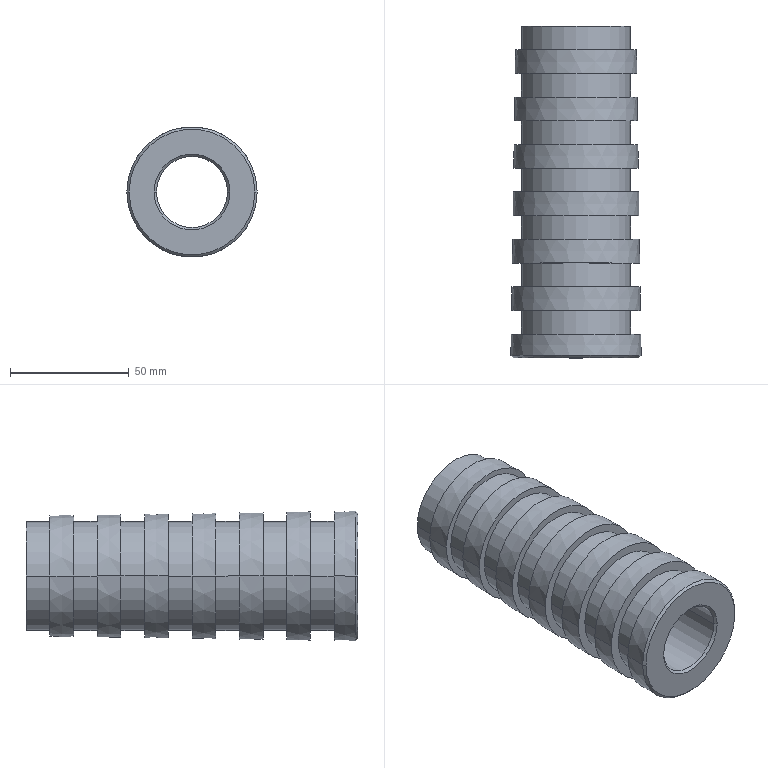Part | SolidWorks | features Revolution 1 | 1 solid | 49 faces | box 54.97 x 140 x 54.97 mm | volume 171748 mm3 | cone 18 | cylinder 16 | plane 15 | commonest cylinder face diameters 46 x14 30 x2
STEP:
#1=CARTESIAN_POINT('',(-26.422,-215.,0.));
#2=VERTEX_POINT('',#1);
#3=CARTESIAN_POINT('',(26.422,-215.,0.));
#4=VERTEX_POINT('',#3);
#5=CARTESIAN_POINT('',(0.,-215.,0.));
#6=DIRECTION('',(0.,1.,0.));
#7=DIRECTION('',(-1.,0.,0.));
#8=AXIS2_PLACEMENT_3D('',#5,#6,#7);
#9=CIRCLE('',#8,26.422);
#10=EDGE_CURVE('',#2,#4,#9,.T.);
#11=ORIENTED_EDGE('',*,*,#10,.F.);
#12=CARTESIAN_POINT('',(-26.576,-225.,0.));
#13=VERTEX_POINT('',#12);
#14=CARTESIAN_POINT('',(-26.422,-215.,0.));
#15=DIRECTION('',(-0.01539,-0.9999,0.));
#16=VECTOR('',#15,1000.);
#17=LINE('',#14,#16);
#18=EDGE_CURVE('',#2,#13,#17,.T.);
#19=ORIENTED_EDGE('',*,*,#18,.T.);
#20=CARTESIAN_POINT('',(26.576,-225.,0.));
#21=VERTEX_POINT('',#20);
#22=CARTESIAN_POINT('',(0.,-225.,0.));
#23=DIRECTION('',(0.,1.,0.));
#24=DIRECTION('',(-1.,0.,0.));
#25=AXIS2_PLACEMENT_3D('',#22,#23,#24);
#26=CIRCLE('',#25,26.576);
#27=EDGE_CURVE('',#13,#21,#26,.T.);
#28=ORIENTED_EDGE('',*,*,#27,.T.);
#29=CARTESIAN_POINT('',(26.422,-215.,0.));
#30=DIRECTION('',(0.01539,-0.9999,0.));
#31=VECTOR('',#30,1000.);
#32=LINE('',#29,#31);
#33=EDGE_CURVE('',#4,#21,#32,.T.);
#34=ORIENTED_EDGE('',*,*,#33,.F.);
#35=EDGE_LOOP('',(#11,#19,#28,#34));
#36=FACE_OUTER_BOUND('',#35,.T.);
#37=CARTESIAN_POINT('',(0.,-215.,0.));
#38=DIRECTION('',(0.,-1.,0.));
#39=DIRECTION('',(1.,0.,0.));
#40=AXIS2_PLACEMENT_3D('',#37,#38,#39);
#41=CONICAL_SURFACE('',#40,26.422,0.0154);
#42=ADVANCED_FACE('',(#36),#41,.T.);
#43=CARTESIAN_POINT('',(-23.,-235.,0.));
#44=VERTEX_POINT('',#43);
#45=CARTESIAN_POINT('',(23.,-235.,0.));
#46=VERTEX_POINT('',#45);
#47=CARTESIAN_POINT('',(0.,-235.,0.));
#48=DIRECTION('',(0.,1.,0.));
#49=DIRECTION('',(-1.,0.,0.));
#50=AXIS2_PLACEMENT_3D('',#47,#48,#49);
#51=CIRCLE('',#50,23.);
#52=EDGE_CURVE('',#44,#46,#51,.T.);
#53=ORIENTED_EDGE('',*,*,#52,.T.);
#54=CARTESIAN_POINT('',(23.,-225.,0.));
#55=VERTEX_POINT('',#54);
#56=CARTESIAN_POINT('',(23.,-285.,0.));
#57=DIRECTION('',(0.,1.,0.));
#58=VECTOR('',#57,1000.);
#59=LINE('',#56,#58);
#60=EDGE_CURVE('',#46,#55,#59,.T.);
#61=ORIENTED_EDGE('',*,*,#60,.T.);
#62=CARTESIAN_POINT('',(-23.,-225.,0.));
#63=VERTEX_POINT('',#62);
#64=CARTESIAN_POINT('',(0.,-225.,0.));
#65=DIRECTION('',(0.,1.,0.));
#66=DIRECTION('',(-1.,0.,0.));
#67=AXIS2_PLACEMENT_3D('',#64,#65,#66);
#68=CIRCLE('',#67,23.);
#69=EDGE_CURVE('',#63,#55,#68,.T.);
#70=ORIENTED_EDGE('',*,*,#69,.F.);
#71=CARTESIAN_POINT('',(-23.,-285.,0.));
#72=DIRECTION('',(0.,1.,0.));
#73=VECTOR('',#72,1000.);
#74=LINE('',#71,#73);
#75=EDGE_CURVE('',#44,#63,#74,.T.);
#76=ORIENTED_EDGE('',*,*,#75,.F.);
#77=EDGE_LOOP('',(#53,#61,#70,#76));
#78=FACE_OUTER_BOUND('',#77,.T.);
#79=CARTESIAN_POINT('',(0.,-285.,0.));
#80=DIRECTION('',(0.,1.,0.));
#81=DIRECTION('',(-1.,0.,0.));
#82=AXIS2_PLACEMENT_3D('',#79,#80,#81);
#83=CYLINDRICAL_SURFACE('',#82,23.);
#84=ADVANCED_FACE('',(#78),#83,.T.);
#85=CARTESIAN_POINT('',(-26.73,-235.,0.));
#86=VERTEX_POINT('',#85);
#87=CARTESIAN_POINT('',(26.73,-235.,0.));
#88=VERTEX_POINT('',#87);
#89=CARTESIAN_POINT('',(0.,-235.,0.));
#90=DIRECTION('',(0.,1.,0.));
#91=DIRECTION('',(-1.,0.,0.));
#92=AXIS2_PLACEMENT_3D('',#89,#90,#91);
#93=CIRCLE('',#92,26.73);
#94=EDGE_CURVE('',#86,#88,#93,.T.);
#95=ORIENTED_EDGE('',*,*,#94,.F.);
#96=CARTESIAN_POINT('',(-26.884,-245.,0.));
#97=VERTEX_POINT('',#96);
#98=CARTESIAN_POINT('',(-26.73,-235.,0.));
#99=DIRECTION('',(-0.01539,-0.9999,0.));
#100=VECTOR('',#99,1000.);
#101=LINE('',#98,#100);
#102=EDGE_CURVE('',#86,#97,#101,.T.);
#103=ORIENTED_EDGE('',*,*,#102,.T.);
#104=CARTESIAN_POINT('',(26.884,-245.,0.));
#105=VERTEX_POINT('',#104);
#106=CARTESIAN_POINT('',(0.,-245.,0.));
#107=DIRECTION('',(0.,1.,0.));
#108=DIRECTION('',(-1.,0.,0.));
#109=AXIS2_PLACEMENT_3D('',#106,#107,#108);
#110=CIRCLE('',#109,26.884);
#111=EDGE_CURVE('',#97,#105,#110,.T.);
#112=ORIENTED_EDGE('',*,*,#111,.T.);
#113=CARTESIAN_POINT('',(26.73,-235.,0.));
#114=DIRECTION('',(0.01539,-0.9999,0.));
#115=VECTOR('',#114,1000.);
#116=LINE('',#113,#115);
#117=EDGE_CURVE('',#88,#105,#116,.T.);
#118=ORIENTED_EDGE('',*,*,#117,.F.);
#119=EDGE_LOOP('',(#95,#103,#112,#118));
#120=FACE_OUTER_BOUND('',#119,.T.);
#121=CARTESIAN_POINT('',(0.,-235.,0.));
#122=DIRECTION('',(0.,-1.,0.));
#123=DIRECTION('',(1.,0.,0.));
#124=AXIS2_PLACEMENT_3D('',#121,#122,#123);
#125=CONICAL_SURFACE('',#124,26.73,0.0154);
#126=ADVANCED_FACE('',(#120),#125,.T.);
#127=CARTESIAN_POINT('',(-23.,-255.,0.));
#128=VERTEX_POINT('',#127);
#129=CARTESIAN_POINT('',(23.,-255.,0.));
#130=VERTEX_POINT('',#129);
#131=CARTESIAN_POINT('',(0.,-255.,0.));
#132=DIRECTION('',(0.,1.,0.));
#133=DIRECTION('',(-1.,0.,0.));
#134=AXIS2_PLACEMENT_3D('',#131,#132,#133);
#135=CIRCLE('',#134,23.);
#136=EDGE_CURVE('',#128,#130,#135,.T.);
#137=ORIENTED_EDGE('',*,*,#136,.T.);
#138=CARTESIAN_POINT('',(23.,-245.,0.));
#139=VERTEX_POINT('',#138);
#140=CARTESIAN_POINT('',(23.,-285.,0.));
#141=DIRECTION('',(0.,1.,0.));
#142=VECTOR('',#141,1000.);
#143=LINE('',#140,#142);
#144=EDGE_CURVE('',#130,#139,#143,.T.);
#145=ORIENTED_EDGE('',*,*,#144,.T.);
#146=CARTESIAN_POINT('',(-23.,-245.,0.));
#147=VERTEX_POINT('',#146);
#148=CARTESIAN_POINT('',(0.,-245.,0.));
#149=DIRECTION('',(0.,1.,0.));
#150=DIRECTION('',(-1.,0.,0.));
#151=AXIS2_PLACEMENT_3D('',#148,#149,#150);
#152=CIRCLE('',#151,23.);
#153=EDGE_CURVE('',#147,#139,#152,.T.);
#154=ORIENTED_EDGE('',*,*,#153,.F.);
#155=CARTESIAN_POINT('',(-23.,-285.,0.));
#156=DIRECTION('',(0.,1.,0.));
#157=VECTOR('',#156,1000.);
#158=LINE('',#155,#157);
#159=EDGE_CURVE('',#128,#147,#158,.T.);
#160=ORIENTED_EDGE('',*,*,#159,.F.);
#161=EDGE_LOOP('',(#137,#145,#154,#160));
#162=FACE_OUTER_BOUND('',#161,.T.);
#163=CARTESIAN_POINT('',(0.,-285.,0.));
#164=DIRECTION('',(0.,1.,0.));
#165=DIRECTION('',(-1.,0.,0.));
#166=AXIS2_PLACEMENT_3D('',#163,#164,#165);
#167=CYLINDRICAL_SURFACE('',#166,23.);
#168=ADVANCED_FACE('',(#162),#167,.T.);
#169=CARTESIAN_POINT('',(-27.038,-255.,0.));
#170=VERTEX_POINT('',#169);
#171=CARTESIAN_POINT('',(27.038,-255.,0.));
#172=VERTEX_POINT('',#171);
#173=CARTESIAN_POINT('',(0.,-255.,0.));
#174=DIRECTION('',(0.,1.,0.));
#175=DIRECTION('',(-1.,0.,0.));
#176=AXIS2_PLACEMENT_3D('',#173,#174,#175);
#177=CIRCLE('',#176,27.038);
#178=EDGE_CURVE('',#170,#172,#177,.T.);
#179=ORIENTED_EDGE('',*,*,#178,.F.);
#180=CARTESIAN_POINT('',(-27.192,-265.,0.));
#181=VERTEX_POINT('',#180);
#182=CARTESIAN_POINT('',(-27.038,-255.,0.));
#183=DIRECTION('',(-0.01539,-0.9999,0.));
#184=VECTOR('',#183,1000.);
#185=LINE('',#182,#184);
#186=EDGE_CURVE('',#170,#181,#185,.T.);
#187=ORIENTED_EDGE('',*,*,#186,.T.);
#188=CARTESIAN_POINT('',(27.192,-265.,0.));
#189=VERTEX_POINT('',#188);
#190=CARTESIAN_POINT('',(0.,-265.,0.));
#191=DIRECTION('',(0.,1.,0.));
#192=DIRECTION('',(-1.,0.,0.));
#193=AXIS2_PLACEMENT_3D('',#190,#191,#192);
#194=CIRCLE('',#193,27.192);
#195=EDGE_CURVE('',#181,#189,#194,.T.);
#196=ORIENTED_EDGE('',*,*,#195,.T.);
#197=CARTESIAN_POINT('',(27.038,-255.,0.));
#198=DIRECTION('',(0.01539,-0.9999,0.));
#199=VECTOR('',#198,1000.);
#200=LINE('',#197,#199);
#201=EDGE_CURVE('',#172,#189,#200,.T.);
#202=ORIENTED_EDGE('',*,*,#201,.F.);
#203=EDGE_LOOP('',(#179,#187,#196,#202));
#204=FACE_OUTER_BOUND('',#203,.T.);
#205=CARTESIAN_POINT('',(0.,-255.,0.));
#206=DIRECTION('',(0.,-1.,0.));
#207=DIRECTION('',(1.,0.,0.));
#208=AXIS2_PLACEMENT_3D('',#205,#206,#207);
#209=CONICAL_SURFACE('',#208,27.038,0.0154);
#210=ADVANCED_FACE('',(#204),#209,.T.);
#211=CARTESIAN_POINT('',(-23.,-275.,0.));
#212=VERTEX_POINT('',#211);
#213=CARTESIAN_POINT('',(23.,-275.,0.));
#214=VERTEX_POINT('',#213);
#215=CARTESIAN_POINT('',(0.,-275.,0.));
#216=DIRECTION('',(0.,1.,0.));
#217=DIRECTION('',(-1.,0.,0.));
#218=AXIS2_PLACEMENT_3D('',#215,#216,#217);
#219=CIRCLE('',#218,23.);
#220=EDGE_CURVE('',#212,#214,#219,.T.);
#221=ORIENTED_EDGE('',*,*,#220,.T.);
#222=CARTESIAN_POINT('',(23.,-265.,0.));
#223=VERTEX_POINT('',#222);
#224=CARTESIAN_POINT('',(23.,-285.,0.));
#225=DIRECTION('',(0.,1.,0.));
#226=VECTOR('',#225,1000.);
#227=LINE('',#224,#226);
#228=EDGE_CURVE('',#214,#223,#227,.T.);
#229=ORIENTED_EDGE('',*,*,#228,.T.);
#230=CARTESIAN_POINT('',(-23.,-265.,0.));
#231=VERTEX_POINT('',#230);
#232=CARTESIAN_POINT('',(0.,-265.,0.));
#233=DIRECTION('',(0.,1.,0.));
#234=DIRECTION('',(-1.,0.,0.));
#235=AXIS2_PLACEMENT_3D('',#232,#233,#234);
#236=CIRCLE('',#235,23.);
#237=EDGE_CURVE('',#231,#223,#236,.T.);
#238=ORIENTED_EDGE('',*,*,#237,.F.);
#239=CARTESIAN_POINT('',(-23.,-285.,0.));
#240=DIRECTION('',(0.,1.,0.));
#241=VECTOR('',#240,1000.);
#242=LINE('',#239,#241);
#243=EDGE_CURVE('',#212,#231,#242,.T.);
#244=ORIENTED_EDGE('',*,*,#243,.F.);
#245=EDGE_LOOP('',(#221,#229,#238,#244));
#246=FACE_OUTER_BOUND('',#245,.T.);
#247=CARTESIAN_POINT('',(0.,-285.,0.));
#248=DIRECTION('',(0.,1.,0.));
#249=DIRECTION('',(-1.,0.,0.));
#250=AXIS2_PLACEMENT_3D('',#247,#248,#249);
#251=CYLINDRICAL_SURFACE('',#250,23.);
#252=ADVANCED_FACE('',(#246),#251,.T.);
#253=CARTESIAN_POINT('',(-27.346,-275.,0.));
#254=VERTEX_POINT('',#253);
#255=CARTESIAN_POINT('',(27.346,-275.,0.));
#256=VERTEX_POINT('',#255);
#257=CARTESIAN_POINT('',(0.,-275.,0.));
#258=DIRECTION('',(0.,1.,0.));
#259=DIRECTION('',(-1.,0.,0.));
#260=AXIS2_PLACEMENT_3D('',#257,#258,#259);
#261=CIRCLE('',#260,27.346);
#262=EDGE_CURVE('',#254,#256,#261,.T.);
#263=ORIENTED_EDGE('',*,*,#262,.F.);
#264=CARTESIAN_POINT('',(-27.485,-284.015,0.));
#265=VERTEX_POINT('',#264);
#266=CARTESIAN_POINT('',(-27.346,-275.,0.));
#267=DIRECTION('',(-0.01539,-0.9999,0.));
#268=VECTOR('',#267,1000.);
#269=LINE('',#266,#268);
#270=EDGE_CURVE('',#254,#265,#269,.T.);
#271=ORIENTED_EDGE('',*,*,#270,.T.);
#272=CARTESIAN_POINT('',(27.485,-284.015,0.));
#273=VERTEX_POINT('',#272);
#274=CARTESIAN_POINT('',(0.,-284.015,0.));
#275=DIRECTION('',(0.,1.,0.));
#276=DIRECTION('',(-1.,0.,0.));
#277=AXIS2_PLACEMENT_3D('',#274,#275,#276);
#278=CIRCLE('',#277,27.485);
#279=EDGE_CURVE('',#265,#273,#278,.T.);
#280=ORIENTED_EDGE('',*,*,#279,.T.);
#281=CARTESIAN_POINT('',(27.346,-275.,0.));
#282=DIRECTION('',(0.01539,-0.9999,0.));
#283=VECTOR('',#282,1000.);
#284=LINE('',#281,#283);
#285=EDGE_CURVE('',#256,#273,#284,.T.);
#286=ORIENTED_EDGE('',*,*,#285,.F.);
#287=EDGE_LOOP('',(#263,#271,#280,#286));
#288=FACE_OUTER_BOUND('',#287,.T.);
#289=CARTESIAN_POINT('',(0.,-275.,0.));
#290=DIRECTION('',(0.,-1.,0.));
#291=DIRECTION('',(1.,0.,0.));
#292=AXIS2_PLACEMENT_3D('',#289,#290,#291);
#293=CONICAL_SURFACE('',#292,27.346,0.0154);
#294=ADVANCED_FACE('',(#288),#293,.T.);
#295=CARTESIAN_POINT('',(-26.5,-285.,0.));
#296=VERTEX_POINT('',#295);
#297=CARTESIAN_POINT('',(26.5,-285.,0.));
#298=VERTEX_POINT('',#297);
#299=CARTESIAN_POINT('',(0.,-285.,0.));
#300=DIRECTION('',(0.,1.,0.));
#301=DIRECTION('',(-1.,0.,0.));
#302=AXIS2_PLACEMENT_3D('',#299,#300,#301);
#303=CIRCLE('',#302,26.5);
#304=EDGE_CURVE('',#296,#298,#303,.T.);
#305=ORIENTED_EDGE('',*,*,#304,.T.);
#306=CARTESIAN_POINT('',(27.485,-284.015,0.));
#307=DIRECTION('',(0.7071,0.7071,0.));
#308=VECTOR('',#307,1000.);
#309=LINE('',#306,#308);
#310=EDGE_CURVE('',#298,#273,#309,.T.);
#311=ORIENTED_EDGE('',*,*,#310,.T.);
#312=ORIENTED_EDGE('',*,*,#279,.F.);
#313=CARTESIAN_POINT('',(-27.485,-284.015,0.));
#314=DIRECTION('',(-0.7071,0.7071,0.));
#315=VECTOR('',#314,1000.);
#316=LINE('',#313,#315);
#317=EDGE_CURVE('',#296,#265,#316,.T.);
#318=ORIENTED_EDGE('',*,*,#317,.F.);
#319=EDGE_LOOP('',(#305,#311,#312,#318));
#320=FACE_OUTER_BOUND('',#319,.T.);
#321=CARTESIAN_POINT('',(0.,-284.015,0.));
#322=DIRECTION('',(0.,1.,0.));
#323=DIRECTION('',(-1.,0.,0.));
#324=AXIS2_PLACEMENT_3D('',#321,#322,#323);
#325=CONICAL_SURFACE('',#324,27.485,0.7854);
#326=ADVANCED_FACE('',(#320),#325,.T.);
#327=CARTESIAN_POINT('',(15.,-284.,0.));
#328=VERTEX_POINT('',#327);
#329=CARTESIAN_POINT('',(-15.,-284.,0.));
#330=VERTEX_POINT('',#329);
#331=CARTESIAN_POINT('',(0.,-284.,0.));
#332=DIRECTION('',(0.,1.,0.));
#333=DIRECTION('',(-1.,0.,0.));
#334=AXIS2_PLACEMENT_3D('',#331,#332,#333);
#335=CIRCLE('',#334,15.);
#336=EDGE_CURVE('',#328,#330,#335,.T.);
#337=ORIENTED_EDGE('',*,*,#336,.T.);
#338=CARTESIAN_POINT('',(-16.,-285.,0.));
#339=VERTEX_POINT('',#338);
#340=CARTESIAN_POINT('',(-16.,-285.,0.));
#341=DIRECTION('',(-0.7071,-0.7071,0.));
#342=VECTOR('',#341,1000.);
#343=LINE('',#340,#342);
#344=EDGE_CURVE('',#330,#339,#343,.T.);
#345=ORIENTED_EDGE('',*,*,#344,.T.);
#346=CARTESIAN_POINT('',(16.,-285.,0.));
#347=VERTEX_POINT('',#346);
#348=CARTESIAN_POINT('',(0.,-285.,0.));
#349=DIRECTION('',(0.,1.,0.));
#350=DIRECTION('',(-1.,0.,0.));
#351=AXIS2_PLACEMENT_3D('',#348,#349,#350);
#352=CIRCLE('',#351,16.);
#353=EDGE_CURVE('',#347,#339,#352,.T.);
#354=ORIENTED_EDGE('',*,*,#353,.F.);
#355=CARTESIAN_POINT('',(16.,-285.,0.));
#356=DIRECTION('',(0.7071,-0.7071,0.));
#357=VECTOR('',#356,1000.);
#358=LINE('',#355,#357);
#359=EDGE_CURVE('',#328,#347,#358,.T.);
#360=ORIENTED_EDGE('',*,*,#359,.F.);
#361=EDGE_LOOP('',(#337,#345,#354,#360));
#362=FACE_OUTER_BOUND('',#361,.T.);
#363=CARTESIAN_POINT('',(0.,-285.,0.));
#364=DIRECTION('',(0.,-1.,0.));
#365=DIRECTION('',(1.,0.,0.));
#366=AXIS2_PLACEMENT_3D('',#363,#364,#365);
#367=CONICAL_SURFACE('',#366,16.,0.7854);
#368=ADVANCED_FACE('',(#362),#367,.F.);
#369=ORIENTED_EDGE('',*,*,#336,.F.);
#370=CARTESIAN_POINT('',(15.,-145.,0.));
#371=VERTEX_POINT('',#370);
#372=CARTESIAN_POINT('',(15.,-285.,0.));
#373=DIRECTION('',(0.,1.,0.));
#374=VECTOR('',#373,1000.);
#375=LINE('',#372,#374);
#376=EDGE_CURVE('',#328,#371,#375,.T.);
#377=ORIENTED_EDGE('',*,*,#376,.T.);
#378=CARTESIAN_POINT('',(-15.,-145.,0.));
#379=VERTEX_POINT('',#378);
#380=CARTESIAN_POINT('',(0.,-145.,0.));
#381=DIRECTION('',(0.,1.,0.));
#382=DIRECTION('',(-1.,0.,0.));
#383=AXIS2_PLACEMENT_3D('',#380,#381,#382);
#384=CIRCLE('',#383,15.);
#385=EDGE_CURVE('',#371,#379,#384,.T.);
#386=ORIENTED_EDGE('',*,*,#385,.T.);
#387=CARTESIAN_POINT('',(-15.,-285.,0.));
#388=DIRECTION('',(0.,1.,0.));
#389=VECTOR('',#388,1000.);
#390=LINE('',#387,#389);
#391=EDGE_CURVE('',#330,#379,#390,.T.);
#392=ORIENTED_EDGE('',*,*,#391,.F.);
#393=EDGE_LOOP('',(#369,#377,#386,#392));
#394=FACE_OUTER_BOUND('',#393,.T.);
#395=CARTESIAN_POINT('',(0.,-285.,0.));
#396=DIRECTION('',(0.,1.,0.));
#397=DIRECTION('',(-1.,0.,0.));
#398=AXIS2_PLACEMENT_3D('',#395,#396,#397);
#399=CYLINDRICAL_SURFACE('',#398,15.);
#400=ADVANCED_FACE('',(#394),#399,.F.);
#401=CARTESIAN_POINT('',(-23.,-155.,0.));
#402=VERTEX_POINT('',#401);
#403=CARTESIAN_POINT('',(23.,-155.,0.));
#404=VERTEX_POINT('',#403);
#405=CARTESIAN_POINT('',(0.,-155.,0.));
#406=DIRECTION('',(0.,1.,0.));
#407=DIRECTION('',(-1.,0.,0.));
#408=AXIS2_PLACEMENT_3D('',#405,#406,#407);
#409=CIRCLE('',#408,23.);
#410=EDGE_CURVE('',#402,#404,#409,.T.);
#411=ORIENTED_EDGE('',*,*,#410,.T.);
#412=CARTESIAN_POINT('',(23.,-145.,0.));
#413=VERTEX_POINT('',#412);
#414=CARTESIAN_POINT('',(23.,-285.,0.));
#415=DIRECTION('',(0.,1.,0.));
#416=VECTOR('',#415,1000.);
#417=LINE('',#414,#416);
#418=EDGE_CURVE('',#404,#413,#417,.T.);
#419=ORIENTED_EDGE('',*,*,#418,.T.);
#420=CARTESIAN_POINT('',(-23.,-145.,0.));
#421=VERTEX_POINT('',#420);
#422=CARTESIAN_POINT('',(0.,-145.,0.));
#423=DIRECTION('',(0.,1.,0.));
#424=DIRECTION('',(-1.,0.,0.));
#425=AXIS2_PLACEMENT_3D('',#422,#423,#424);
#426=CIRCLE('',#425,23.);
#427=EDGE_CURVE('',#421,#413,#426,.T.);
#428=ORIENTED_EDGE('',*,*,#427,.F.);
#429=CARTESIAN_POINT('',(-23.,-285.,0.));
#430=DIRECTION('',(0.,1.,0.));
#431=VECTOR('',#430,1000.);
#432=LINE('',#429,#431);
#433=EDGE_CURVE('',#402,#421,#432,.T.);
#434=ORIENTED_EDGE('',*,*,#433,.F.);
#435=EDGE_LOOP('',(#411,#419,#428,#434));
#436=FACE_OUTER_BOUND('',#435,.T.);
#437=CARTESIAN_POINT('',(0.,-285.,0.));
#438=DIRECTION('',(0.,1.,0.));
#439=DIRECTION('',(-1.,0.,0.));
#440=AXIS2_PLACEMENT_3D('',#437,#438,#439);
#441=CYLINDRICAL_SURFACE('',#440,23.);
#442=ADVANCED_FACE('',(#436),#441,.T.);
#443=CARTESIAN_POINT('',(-25.498,-155.,0.));
#444=VERTEX_POINT('',#443);
#445=CARTESIAN_POINT('',(25.498,-155.,0.));
#446=VERTEX_POINT('',#445);
#447=CARTESIAN_POINT('',(0.,-155.,0.));
#448=DIRECTION('',(0.,1.,0.));
#449=DIRECTION('',(-1.,0.,0.));
#450=AXIS2_PLACEMENT_3D('',#447,#448,#449);
#451=CIRCLE('',#450,25.498);
#452=EDGE_CURVE('',#444,#446,#451,.T.);
#453=ORIENTED_EDGE('',*,*,#452,.F.);
#454=CARTESIAN_POINT('',(-25.652,-165.,0.));
#455=VERTEX_POINT('',#454);
#456=CARTESIAN_POINT('',(-25.498,-155.,0.));
#457=DIRECTION('',(-0.01539,-0.9999,0.));
#458=VECTOR('',#457,1000.);
#459=LINE('',#456,#458);
#460=EDGE_CURVE('',#444,#455,#459,.T.);
#461=ORIENTED_EDGE('',*,*,#460,.T.);
#462=CARTESIAN_POINT('',(25.652,-165.,0.));
#463=VERTEX_POINT('',#462);
#464=CARTESIAN_POINT('',(0.,-165.,0.));
#465=DIRECTION('',(0.,1.,0.));
#466=DIRECTION('',(-1.,0.,0.));
#467=AXIS2_PLACEMENT_3D('',#464,#465,#466);
#468=CIRCLE('',#467,25.652);
#469=EDGE_CURVE('',#455,#463,#468,.T.);
#470=ORIENTED_EDGE('',*,*,#469,.T.);
#471=CARTESIAN_POINT('',(25.498,-155.,0.));
#472=DIRECTION('',(0.01539,-0.9999,0.));
#473=VECTOR('',#472,1000.);
#474=LINE('',#471,#473);
#475=EDGE_CURVE('',#446,#463,#474,.T.);
#476=ORIENTED_EDGE('',*,*,#475,.F.);
#477=EDGE_LOOP('',(#453,#461,#470,#476));
#478=FACE_OUTER_BOUND('',#477,.T.);
#479=CARTESIAN_POINT('',(0.,-155.,0.));
#480=DIRECTION('',(0.,-1.,0.));
#481=DIRECTION('',(1.,0.,0.));
#482=AXIS2_PLACEMENT_3D('',#479,#480,#481);
#483=CONICAL_SURFACE('',#482,25.498,0.0154);
#484=ADVANCED_FACE('',(#478),#483,.T.);
#485=CARTESIAN_POINT('',(-23.,-175.,0.));
#486=VERTEX_POINT('',#485);
#487=CARTESIAN_POINT('',(23.,-175.,0.));
#488=VERTEX_POINT('',#487);
#489=CARTESIAN_POINT('',(0.,-175.,0.));
#490=DIRECTION('',(0.,1.,0.));
#491=DIRECTION('',(-1.,0.,0.));
#492=AXIS2_PLACEMENT_3D('',#489,#490,#491);
#493=CIRCLE('',#492,23.);
#494=EDGE_CURVE('',#486,#488,#493,.T.);
#495=ORIENTED_EDGE('',*,*,#494,.T.);
#496=CARTESIAN_POINT('',(23.,-165.,0.));
#497=VERTEX_POINT('',#496);
#498=CARTESIAN_POINT('',(23.,-285.,0.));
#499=DIRECTION('',(0.,1.,0.));
#500=VECTOR('',#499,1000.);
#501=LINE('',#498,#500);
#502=EDGE_CURVE('',#488,#497,#501,.T.);
#503=ORIENTED_EDGE('',*,*,#502,.T.);
#504=CARTESIAN_POINT('',(-23.,-165.,0.));
#505=VERTEX_POINT('',#504);
#506=CARTESIAN_POINT('',(0.,-165.,0.));
#507=DIRECTION('',(0.,1.,0.));
#508=DIRECTION('',(-1.,0.,0.));
#509=AXIS2_PLACEMENT_3D('',#506,#507,#508);
#510=CIRCLE('',#509,23.);
#511=EDGE_CURVE('',#505,#497,#510,.T.);
#512=ORIENTED_EDGE('',*,*,#511,.F.);
#513=CARTESIAN_POINT('',(-23.,-285.,0.));
#514=DIRECTION('',(0.,1.,0.));
#515=VECTOR('',#514,1000.);
#516=LINE('',#513,#515);
#517=EDGE_CURVE('',#486,#505,#516,.T.);
#518=ORIENTED_EDGE('',*,*,#517,.F.);
#519=EDGE_LOOP('',(#495,#503,#512,#518));
#520=FACE_OUTER_BOUND('',#519,.T.);
#521=CARTESIAN_POINT('',(0.,-285.,0.));
#522=DIRECTION('',(0.,1.,0.));
#523=DIRECTION('',(-1.,0.,0.));
#524=AXIS2_PLACEMENT_3D('',#521,#522,#523);
#525=CYLINDRICAL_SURFACE('',#524,23.);
#526=ADVANCED_FACE('',(#520),#525,.T.);
#527=CARTESIAN_POINT('',(-25.806,-175.,0.));
#528=VERTEX_POINT('',#527);
#529=CARTESIAN_POINT('',(25.806,-175.,0.));
#530=VERTEX_POINT('',#529);
#531=CARTESIAN_POINT('',(0.,-175.,0.));
#532=DIRECTION('',(0.,1.,0.));
#533=DIRECTION('',(-1.,0.,0.));
#534=AXIS2_PLACEMENT_3D('',#531,#532,#533);
#535=CIRCLE('',#534,25.806);
#536=EDGE_CURVE('',#528,#530,#535,.T.);
#537=ORIENTED_EDGE('',*,*,#536,.F.);
#538=CARTESIAN_POINT('',(-25.96,-185.,0.));
#539=VERTEX_POINT('',#538);
#540=CARTESIAN_POINT('',(-25.806,-175.,0.));
#541=DIRECTION('',(-0.01539,-0.9999,0.));
#542=VECTOR('',#541,1000.);
#543=LINE('',#540,#542);
#544=EDGE_CURVE('',#528,#539,#543,.T.);
#545=ORIENTED_EDGE('',*,*,#544,.T.);
#546=CARTESIAN_POINT('',(25.96,-185.,0.));
#547=VERTEX_POINT('',#546);
#548=CARTESIAN_POINT('',(0.,-185.,0.));
#549=DIRECTION('',(0.,1.,0.));
#550=DIRECTION('',(-1.,0.,0.));
#551=AXIS2_PLACEMENT_3D('',#548,#549,#550);
#552=CIRCLE('',#551,25.96);
#553=EDGE_CURVE('',#539,#547,#552,.T.);
#554=ORIENTED_EDGE('',*,*,#553,.T.);
#555=CARTESIAN_POINT('',(25.806,-175.,0.));
#556=DIRECTION('',(0.01539,-0.9999,0.));
#557=VECTOR('',#556,1000.);
#558=LINE('',#555,#557);
#559=EDGE_CURVE('',#530,#547,#558,.T.);
#560=ORIENTED_EDGE('',*,*,#559,.F.);
#561=EDGE_LOOP('',(#537,#545,#554,#560));
#562=FACE_OUTER_BOUND('',#561,.T.);
#563=CARTESIAN_POINT('',(0.,-175.,0.));
#564=DIRECTION('',(0.,-1.,0.));
#565=DIRECTION('',(1.,0.,0.));
#566=AXIS2_PLACEMENT_3D('',#563,#564,#565);
#567=CONICAL_SURFACE('',#566,25.806,0.0154);
#568=ADVANCED_FACE('',(#562),#567,.T.);
#569=CARTESIAN_POINT('',(-23.,-195.,0.));
#570=VERTEX_POINT('',#569);
#571=CARTESIAN_POINT('',(23.,-195.,0.));
#572=VERTEX_POINT('',#571);
#573=CARTESIAN_POINT('',(0.,-195.,0.));
#574=DIRECTION('',(0.,1.,0.));
#575=DIRECTION('',(-1.,0.,0.));
#576=AXIS2_PLACEMENT_3D('',#573,#574,#575);
#577=CIRCLE('',#576,23.);
#578=EDGE_CURVE('',#570,#572,#577,.T.);
#579=ORIENTED_EDGE('',*,*,#578,.T.);
#580=CARTESIAN_POINT('',(23.,-185.,0.));
#581=VERTEX_POINT('',#580);
#582=CARTESIAN_POINT('',(23.,-285.,0.));
#583=DIRECTION('',(0.,1.,0.));
#584=VECTOR('',#583,1000.);
#585=LINE('',#582,#584);
#586=EDGE_CURVE('',#572,#581,#585,.T.);
#587=ORIENTED_EDGE('',*,*,#586,.T.);
#588=CARTESIAN_POINT('',(-23.,-185.,0.));
#589=VERTEX_POINT('',#588);
#590=CARTESIAN_POINT('',(0.,-185.,0.));
#591=DIRECTION('',(0.,1.,0.));
#592=DIRECTION('',(-1.,0.,0.));
#593=AXIS2_PLACEMENT_3D('',#590,#591,#592);
#594=CIRCLE('',#593,23.);
#595=EDGE_CURVE('',#589,#581,#594,.T.);
#596=ORIENTED_EDGE('',*,*,#595,.F.);
#597=CARTESIAN_POINT('',(-23.,-285.,0.));
#598=DIRECTION('',(0.,1.,0.));
#599=VECTOR('',#598,1000.);
#600=LINE('',#597,#599);
#601=EDGE_CURVE('',#570,#589,#600,.T.);
#602=ORIENTED_EDGE('',*,*,#601,.F.);
#603=EDGE_LOOP('',(#579,#587,#596,#602));
#604=FACE_OUTER_BOUND('',#603,.T.);
#605=CARTESIAN_POINT('',(0.,-285.,0.));
#606=DIRECTION('',(0.,1.,0.));
#607=DIRECTION('',(-1.,0.,0.));
#608=AXIS2_PLACEMENT_3D('',#605,#606,#607);
#609=CYLINDRICAL_SURFACE('',#608,23.);
#610=ADVANCED_FACE('',(#604),#609,.T.);
#611=CARTESIAN_POINT('',(-26.114,-195.,0.));
#612=VERTEX_POINT('',#611);
#613=CARTESIAN_POINT('',(26.114,-195.,0.));
#614=VERTEX_POINT('',#613);
#615=CARTESIAN_POINT('',(0.,-195.,0.));
#616=DIRECTION('',(0.,1.,0.));
#617=DIRECTION('',(-1.,0.,0.));
#618=AXIS2_PLACEMENT_3D('',#615,#616,#617);
#619=CIRCLE('',#618,26.114);
#620=EDGE_CURVE('',#612,#614,#619,.T.);
#621=ORIENTED_EDGE('',*,*,#620,.F.);
#622=CARTESIAN_POINT('',(-26.268,-205.,0.));
#623=VERTEX_POINT('',#622);
#624=CARTESIAN_POINT('',(-26.114,-195.,0.));
#625=DIRECTION('',(-0.01539,-0.9999,0.));
#626=VECTOR('',#625,1000.);
#627=LINE('',#624,#626);
#628=EDGE_CURVE('',#612,#623,#627,.T.);
#629=ORIENTED_EDGE('',*,*,#628,.T.);
#630=CARTESIAN_POINT('',(26.268,-205.,0.));
#631=VERTEX_POINT('',#630);
#632=CARTESIAN_POINT('',(0.,-205.,0.));
#633=DIRECTION('',(0.,1.,0.));
#634=DIRECTION('',(-1.,0.,0.));
#635=AXIS2_PLACEMENT_3D('',#632,#633,#634);
#636=CIRCLE('',#635,26.268);
#637=EDGE_CURVE('',#623,#631,#636,.T.);
#638=ORIENTED_EDGE('',*,*,#637,.T.);
#639=CARTESIAN_POINT('',(26.114,-195.,0.));
#640=DIRECTION('',(0.01539,-0.9999,0.));
#641=VECTOR('',#640,1000.);
#642=LINE('',#639,#641);
#643=EDGE_CURVE('',#614,#631,#642,.T.);
#644=ORIENTED_EDGE('',*,*,#643,.F.);
#645=EDGE_LOOP('',(#621,#629,#638,#644));
#646=FACE_OUTER_BOUND('',#645,.T.);
#647=CARTESIAN_POINT('',(0.,-195.,0.));
#648=DIRECTION('',(0.,-1.,0.));
#649=DIRECTION('',(1.,0.,0.));
#650=AXIS2_PLACEMENT_3D('',#647,#648,#649);
#651=CONICAL_SURFACE('',#650,26.114,0.0154);
#652=ADVANCED_FACE('',(#646),#651,.T.);
#653=CARTESIAN_POINT('',(-23.,-215.,0.));
#654=VERTEX_POINT('',#653);
#655=CARTESIAN_POINT('',(23.,-215.,0.));
#656=VERTEX_POINT('',#655);
#657=CARTESIAN_POINT('',(0.,-215.,0.));
#658=DIRECTION('',(0.,1.,0.));
#659=DIRECTION('',(-1.,0.,0.));
#660=AXIS2_PLACEMENT_3D('',#657,#658,#659);
#661=CIRCLE('',#660,23.);
#662=EDGE_CURVE('',#654,#656,#661,.T.);
#663=ORIENTED_EDGE('',*,*,#662,.T.);
#664=CARTESIAN_POINT('',(23.,-205.,0.));
#665=VERTEX_POINT('',#664);
#666=CARTESIAN_POINT('',(23.,-285.,0.));
#667=DIRECTION('',(0.,1.,0.));
#668=VECTOR('',#667,1000.);
#669=LINE('',#666,#668);
#670=EDGE_CURVE('',#656,#665,#669,.T.);
#671=ORIENTED_EDGE('',*,*,#670,.T.);
#672=CARTESIAN_POINT('',(-23.,-205.,0.));
#673=VERTEX_POINT('',#672);
#674=CARTESIAN_POINT('',(0.,-205.,0.));
#675=DIRECTION('',(0.,1.,0.));
#676=DIRECTION('',(-1.,0.,0.));
#677=AXIS2_PLACEMENT_3D('',#674,#675,#676);
#678=CIRCLE('',#677,23.);
#679=EDGE_CURVE('',#673,#665,#678,.T.);
#680=ORIENTED_EDGE('',*,*,#679,.F.);
#681=CARTESIAN_POINT('',(-23.,-285.,0.));
#682=DIRECTION('',(0.,1.,0.));
#683=VECTOR('',#682,1000.);
#684=LINE('',#681,#683);
#685=EDGE_CURVE('',#654,#673,#684,.T.);
#686=ORIENTED_EDGE('',*,*,#685,.F.);
#687=EDGE_LOOP('',(#663,#671,#680,#686));
#688=FACE_OUTER_BOUND('',#687,.T.);
#689=CARTESIAN_POINT('',(0.,-285.,0.));
#690=DIRECTION('',(0.,1.,0.));
#691=DIRECTION('',(-1.,0.,0.));
#692=AXIS2_PLACEMENT_3D('',#689,#690,#691);
#693=CYLINDRICAL_SURFACE('',#692,23.);
#694=ADVANCED_FACE('',(#688),#693,.T.);
#695=ORIENTED_EDGE('',*,*,#670,.F.);
#696=CARTESIAN_POINT('',(0.,-215.,0.));
#697=DIRECTION('',(0.,1.,0.));
#698=DIRECTION('',(-1.,0.,0.));
#699=AXIS2_PLACEMENT_3D('',#696,#697,#698);
#700=CIRCLE('',#699,23.);
#701=EDGE_CURVE('',#656,#654,#700,.T.);
#702=ORIENTED_EDGE('',*,*,#701,.T.);
#703=ORIENTED_EDGE('',*,*,#685,.T.);
#704=CARTESIAN_POINT('',(0.,-205.,0.));
#705=DIRECTION('',(0.,1.,0.));
#706=DIRECTION('',(-1.,0.,0.));
#707=AXIS2_PLACEMENT_3D('',#704,#705,#706);
#708=CIRCLE('',#707,23.);
#709=EDGE_CURVE('',#665,#673,#708,.T.);
#710=ORIENTED_EDGE('',*,*,#709,.F.);
#711=EDGE_LOOP('',(#695,#702,#703,#710));
#712=FACE_OUTER_BOUND('',#711,.T.);
#713=CARTESIAN_POINT('',(0.,-285.,0.));
#714=DIRECTION('',(0.,1.,0.));
#715=DIRECTION('',(-1.,0.,0.));
#716=AXIS2_PLACEMENT_3D('',#713,#714,#715);
#717=CYLINDRICAL_SURFACE('',#716,23.);
#718=ADVANCED_FACE('',(#712),#717,.T.);
#719=ORIENTED_EDGE('',*,*,#679,.T.);
#720=ORIENTED_EDGE('',*,*,#709,.T.);
#721=EDGE_LOOP('',(#719,#720));
#722=FACE_BOUND('',#721,.T.);
#723=CARTESIAN_POINT('',(0.,-205.,0.));
#724=DIRECTION('',(0.,1.,0.));
#725=DIRECTION('',(-1.,0.,0.));
#726=AXIS2_PLACEMENT_3D('',#723,#724,#725);
#727=CIRCLE('',#726,26.268);
#728=EDGE_CURVE('',#631,#623,#727,.T.);
#729=ORIENTED_EDGE('',*,*,#728,.F.);
#730=ORIENTED_EDGE('',*,*,#637,.F.);
#731=EDGE_LOOP('',(#729,#730));
#732=FACE_OUTER_BOUND('',#731,.T.);
#733=CARTESIAN_POINT('',(26.268,-205.,0.));
#734=DIRECTION('',(0.,-1.,0.));
#735=DIRECTION('',(1.,0.,0.));
#736=AXIS2_PLACEMENT_3D('',#733,#734,#735);
#737=PLANE('',#736);
#738=ADVANCED_FACE('',(#722,#732),#737,.T.);
#739=ORIENTED_EDGE('',*,*,#628,.F.);
#740=CARTESIAN_POINT('',(0.,-195.,0.));
#741=DIRECTION('',(0.,1.,0.));
#742=DIRECTION('',(-1.,0.,0.));
#743=AXIS2_PLACEMENT_3D('',#740,#741,#742);
#744=CIRCLE('',#743,26.114);
#745=EDGE_CURVE('',#614,#612,#744,.T.);
#746=ORIENTED_EDGE('',*,*,#745,.F.);
#747=ORIENTED_EDGE('',*,*,#643,.T.);
#748=ORIENTED_EDGE('',*,*,#728,.T.);
#749=EDGE_LOOP('',(#739,#746,#747,#748));
#750=FACE_OUTER_BOUND('',#749,.T.);
#751=CARTESIAN_POINT('',(0.,-195.,0.));
#752=DIRECTION('',(0.,-1.,0.));
#753=DIRECTION('',(1.,0.,0.));
#754=AXIS2_PLACEMENT_3D('',#751,#752,#753);
#755=CONICAL_SURFACE('',#754,26.114,0.0154);
#756=ADVANCED_FACE('',(#750),#755,.T.);
#757=ORIENTED_EDGE('',*,*,#745,.T.);
#758=ORIENTED_EDGE('',*,*,#620,.T.);
#759=EDGE_LOOP('',(#757,#758));
#760=FACE_OUTER_BOUND('',#759,.T.);
#761=ORIENTED_EDGE('',*,*,#578,.F.);
#762=CARTESIAN_POINT('',(0.,-195.,0.));
#763=DIRECTION('',(0.,1.,0.));
#764=DIRECTION('',(-1.,0.,0.));
#765=AXIS2_PLACEMENT_3D('',#762,#763,#764);
#766=CIRCLE('',#765,23.);
#767=EDGE_CURVE('',#572,#570,#766,.T.);
#768=ORIENTED_EDGE('',*,*,#767,.F.);
#769=EDGE_LOOP('',(#761,#768));
#770=FACE_BOUND('',#769,.T.);
#771=CARTESIAN_POINT('',(23.,-195.,0.));
#772=DIRECTION('',(0.,1.,0.));
#773=DIRECTION('',(-1.,0.,0.));
#774=AXIS2_PLACEMENT_3D('',#771,#772,#773);
#775=PLANE('',#774);
#776=ADVANCED_FACE('',(#760,#770),#775,.T.);
#777=ORIENTED_EDGE('',*,*,#586,.F.);
#778=ORIENTED_EDGE('',*,*,#767,.T.);
#779=ORIENTED_EDGE('',*,*,#601,.T.);
#780=CARTESIAN_POINT('',(0.,-185.,0.));
#781=DIRECTION('',(0.,1.,0.));
#782=DIRECTION('',(-1.,0.,0.));
#783=AXIS2_PLACEMENT_3D('',#780,#781,#782);
#784=CIRCLE('',#783,23.);
#785=EDGE_CURVE('',#581,#589,#784,.T.);
#786=ORIENTED_EDGE('',*,*,#785,.F.);
#787=EDGE_LOOP('',(#777,#778,#779,#786));
#788=FACE_OUTER_BOUND('',#787,.T.);
#789=CARTESIAN_POINT('',(0.,-285.,0.));
#790=DIRECTION('',(0.,1.,0.));
#791=DIRECTION('',(-1.,0.,0.));
#792=AXIS2_PLACEMENT_3D('',#789,#790,#791);
#793=CYLINDRICAL_SURFACE('',#792,23.);
#794=ADVANCED_FACE('',(#788),#793,.T.);
#795=ORIENTED_EDGE('',*,*,#595,.T.);
#796=ORIENTED_EDGE('',*,*,#785,.T.);
#797=EDGE_LOOP('',(#795,#796));
#798=FACE_BOUND('',#797,.T.);
#799=CARTESIAN_POINT('',(0.,-185.,0.));
#800=DIRECTION('',(0.,1.,0.));
#801=DIRECTION('',(-1.,0.,0.));
#802=AXIS2_PLACEMENT_3D('',#799,#800,#801);
#803=CIRCLE('',#802,25.96);
#804=EDGE_CURVE('',#547,#539,#803,.T.);
#805=ORIENTED_EDGE('',*,*,#804,.F.);
#806=ORIENTED_EDGE('',*,*,#553,.F.);
#807=EDGE_LOOP('',(#805,#806));
#808=FACE_OUTER_BOUND('',#807,.T.);
#809=CARTESIAN_POINT('',(25.96,-185.,0.));
#810=DIRECTION('',(0.,-1.,0.));
#811=DIRECTION('',(1.,0.,0.));
#812=AXIS2_PLACEMENT_3D('',#809,#810,#811);
#813=PLANE('',#812);
#814=ADVANCED_FACE('',(#798,#808),#813,.T.);
#815=ORIENTED_EDGE('',*,*,#544,.F.);
#816=CARTESIAN_POINT('',(0.,-175.,0.));
#817=DIRECTION('',(0.,1.,0.));
#818=DIRECTION('',(-1.,0.,0.));
#819=AXIS2_PLACEMENT_3D('',#816,#817,#818);
#820=CIRCLE('',#819,25.806);
#821=EDGE_CURVE('',#530,#528,#820,.T.);
#822=ORIENTED_EDGE('',*,*,#821,.F.);
#823=ORIENTED_EDGE('',*,*,#559,.T.);
#824=ORIENTED_EDGE('',*,*,#804,.T.);
#825=EDGE_LOOP('',(#815,#822,#823,#824));
#826=FACE_OUTER_BOUND('',#825,.T.);
#827=CARTESIAN_POINT('',(0.,-175.,0.));
#828=DIRECTION('',(0.,-1.,0.));
#829=DIRECTION('',(1.,0.,0.));
#830=AXIS2_PLACEMENT_3D('',#827,#828,#829);
#831=CONICAL_SURFACE('',#830,25.806,0.0154);
#832=ADVANCED_FACE('',(#826),#831,.T.);
#833=ORIENTED_EDGE('',*,*,#821,.T.);
#834=ORIENTED_EDGE('',*,*,#536,.T.);
#835=EDGE_LOOP('',(#833,#834));
#836=FACE_OUTER_BOUND('',#835,.T.);
#837=ORIENTED_EDGE('',*,*,#494,.F.);
#838=CARTESIAN_POINT('',(0.,-175.,0.));
#839=DIRECTION('',(0.,1.,0.));
#840=DIRECTION('',(-1.,0.,0.));
#841=AXIS2_PLACEMENT_3D('',#838,#839,#840);
#842=CIRCLE('',#841,23.);
#843=EDGE_CURVE('',#488,#486,#842,.T.);
#844=ORIENTED_EDGE('',*,*,#843,.F.);
#845=EDGE_LOOP('',(#837,#844));
#846=FACE_BOUND('',#845,.T.);
#847=CARTESIAN_POINT('',(23.,-175.,0.));
#848=DIRECTION('',(0.,1.,0.));
#849=DIRECTION('',(-1.,0.,0.));
#850=AXIS2_PLACEMENT_3D('',#847,#848,#849);
#851=PLANE('',#850);
#852=ADVANCED_FACE('',(#836,#846),#851,.T.);
#853=ORIENTED_EDGE('',*,*,#502,.F.);
#854=ORIENTED_EDGE('',*,*,#843,.T.);
#855=ORIENTED_EDGE('',*,*,#517,.T.);
#856=CARTESIAN_POINT('',(0.,-165.,0.));
#857=DIRECTION('',(0.,1.,0.));
#858=DIRECTION('',(-1.,0.,0.));
#859=AXIS2_PLACEMENT_3D('',#856,#857,#858);
#860=CIRCLE('',#859,23.);
#861=EDGE_CURVE('',#497,#505,#860,.T.);
#862=ORIENTED_EDGE('',*,*,#861,.F.);
#863=EDGE_LOOP('',(#853,#854,#855,#862));
#864=FACE_OUTER_BOUND('',#863,.T.);
#865=CARTESIAN_POINT('',(0.,-285.,0.));
#866=DIRECTION('',(0.,1.,0.));
#867=DIRECTION('',(-1.,0.,0.));
#868=AXIS2_PLACEMENT_3D('',#865,#866,#867);
#869=CYLINDRICAL_SURFACE('',#868,23.);
#870=ADVANCED_FACE('',(#864),#869,.T.);
#871=ORIENTED_EDGE('',*,*,#511,.T.);
#872=ORIENTED_EDGE('',*,*,#861,.T.);
#873=EDGE_LOOP('',(#871,#872));
#874=FACE_BOUND('',#873,.T.);
#875=CARTESIAN_POINT('',(0.,-165.,0.));
#876=DIRECTION('',(0.,1.,0.));
#877=DIRECTION('',(-1.,0.,0.));
#878=AXIS2_PLACEMENT_3D('',#875,#876,#877);
#879=CIRCLE('',#878,25.652);
#880=EDGE_CURVE('',#463,#455,#879,.T.);
#881=ORIENTED_EDGE('',*,*,#880,.F.);
#882=ORIENTED_EDGE('',*,*,#469,.F.);
#883=EDGE_LOOP('',(#881,#882));
#884=FACE_OUTER_BOUND('',#883,.T.);
#885=CARTESIAN_POINT('',(25.652,-165.,0.));
#886=DIRECTION('',(0.,-1.,0.));
#887=DIRECTION('',(1.,0.,0.));
#888=AXIS2_PLACEMENT_3D('',#885,#886,#887);
#889=PLANE('',#888);
#890=ADVANCED_FACE('',(#874,#884),#889,.T.);
#891=ORIENTED_EDGE('',*,*,#460,.F.);
#892=CARTESIAN_POINT('',(0.,-155.,0.));
#893=DIRECTION('',(0.,1.,0.));
#894=DIRECTION('',(-1.,0.,0.));
#895=AXIS2_PLACEMENT_3D('',#892,#893,#894);
#896=CIRCLE('',#895,25.498);
#897=EDGE_CURVE('',#446,#444,#896,.T.);
#898=ORIENTED_EDGE('',*,*,#897,.F.);
#899=ORIENTED_EDGE('',*,*,#475,.T.);
#900=ORIENTED_EDGE('',*,*,#880,.T.);
#901=EDGE_LOOP('',(#891,#898,#899,#900));
#902=FACE_OUTER_BOUND('',#901,.T.);
#903=CARTESIAN_POINT('',(0.,-155.,0.));
#904=DIRECTION('',(0.,-1.,0.));
#905=DIRECTION('',(1.,0.,0.));
#906=AXIS2_PLACEMENT_3D('',#903,#904,#905);
#907=CONICAL_SURFACE('',#906,25.498,0.0154);
#908=ADVANCED_FACE('',(#902),#907,.T.);
#909=ORIENTED_EDGE('',*,*,#897,.T.);
#910=ORIENTED_EDGE('',*,*,#452,.T.);
#911=EDGE_LOOP('',(#909,#910));
#912=FACE_OUTER_BOUND('',#911,.T.);
#913=ORIENTED_EDGE('',*,*,#410,.F.);
#914=CARTESIAN_POINT('',(0.,-155.,0.));
#915=DIRECTION('',(0.,1.,0.));
#916=DIRECTION('',(-1.,0.,0.));
#917=AXIS2_PLACEMENT_3D('',#914,#915,#916);
#918=CIRCLE('',#917,23.);
#919=EDGE_CURVE('',#404,#402,#918,.T.);
#920=ORIENTED_EDGE('',*,*,#919,.F.);
#921=EDGE_LOOP('',(#913,#920));
#922=FACE_BOUND('',#921,.T.);
#923=CARTESIAN_POINT('',(23.,-155.,0.));
#924=DIRECTION('',(0.,1.,0.));
#925=DIRECTION('',(-1.,0.,0.));
#926=AXIS2_PLACEMENT_3D('',#923,#924,#925);
#927=PLANE('',#926);
#928=ADVANCED_FACE('',(#912,#922),#927,.T.);
#929=ORIENTED_EDGE('',*,*,#418,.F.);
#930=ORIENTED_EDGE('',*,*,#919,.T.);
#931=ORIENTED_EDGE('',*,*,#433,.T.);
#932=CARTESIAN_POINT('',(0.,-145.,0.));
#933=DIRECTION('',(0.,1.,0.));
#934=DIRECTION('',(-1.,0.,0.));
#935=AXIS2_PLACEMENT_3D('',#932,#933,#934);
#936=CIRCLE('',#935,23.);
#937=EDGE_CURVE('',#413,#421,#936,.T.);
#938=ORIENTED_EDGE('',*,*,#937,.F.);
#939=EDGE_LOOP('',(#929,#930,#931,#938));
#940=FACE_OUTER_BOUND('',#939,.T.);
#941=CARTESIAN_POINT('',(0.,-285.,0.));
#942=DIRECTION('',(0.,1.,0.));
#943=DIRECTION('',(-1.,0.,0.));
#944=AXIS2_PLACEMENT_3D('',#941,#942,#943);
#945=CYLINDRICAL_SURFACE('',#944,23.);
#946=ADVANCED_FACE('',(#940),#945,.T.);
#947=ORIENTED_EDGE('',*,*,#427,.T.);
#948=ORIENTED_EDGE('',*,*,#937,.T.);
#949=EDGE_LOOP('',(#947,#948));
#950=FACE_OUTER_BOUND('',#949,.T.);
#951=CARTESIAN_POINT('',(0.,-145.,0.));
#952=DIRECTION('',(0.,1.,0.));
#953=DIRECTION('',(-1.,0.,0.));
#954=AXIS2_PLACEMENT_3D('',#951,#952,#953);
#955=CIRCLE('',#954,15.);
#956=EDGE_CURVE('',#379,#371,#955,.T.);
#957=ORIENTED_EDGE('',*,*,#956,.F.);
#958=ORIENTED_EDGE('',*,*,#385,.F.);
#959=EDGE_LOOP('',(#957,#958));
#960=FACE_BOUND('',#959,.T.);
#961=CARTESIAN_POINT('',(15.,-145.,0.));
#962=DIRECTION('',(0.,1.,0.));
#963=DIRECTION('',(-1.,0.,0.));
#964=AXIS2_PLACEMENT_3D('',#961,#962,#963);
#965=PLANE('',#964);
#966=ADVANCED_FACE('',(#950,#960),#965,.T.);
#967=ORIENTED_EDGE('',*,*,#376,.F.);
#968=CARTESIAN_POINT('',(0.,-284.,0.));
#969=DIRECTION('',(0.,1.,0.));
#970=DIRECTION('',(-1.,0.,0.));
#971=AXIS2_PLACEMENT_3D('',#968,#969,#970);
#972=CIRCLE('',#971,15.);
#973=EDGE_CURVE('',#330,#328,#972,.T.);
#974=ORIENTED_EDGE('',*,*,#973,.F.);
#975=ORIENTED_EDGE('',*,*,#391,.T.);
#976=ORIENTED_EDGE('',*,*,#956,.T.);
#977=EDGE_LOOP('',(#967,#974,#975,#976));
#978=FACE_OUTER_BOUND('',#977,.T.);
#979=CARTESIAN_POINT('',(0.,-285.,0.));
#980=DIRECTION('',(0.,1.,0.));
#981=DIRECTION('',(-1.,0.,0.));
#982=AXIS2_PLACEMENT_3D('',#979,#980,#981);
#983=CYLINDRICAL_SURFACE('',#982,15.);
#984=ADVANCED_FACE('',(#978),#983,.F.);
#985=ORIENTED_EDGE('',*,*,#344,.F.);
#986=ORIENTED_EDGE('',*,*,#973,.T.);
#987=ORIENTED_EDGE('',*,*,#359,.T.);
#988=CARTESIAN_POINT('',(0.,-285.,0.));
#989=DIRECTION('',(0.,1.,0.));
#990=DIRECTION('',(-1.,0.,0.));
#991=AXIS2_PLACEMENT_3D('',#988,#989,#990);
#992=CIRCLE('',#991,16.);
#993=EDGE_CURVE('',#339,#347,#992,.T.);
#994=ORIENTED_EDGE('',*,*,#993,.F.);
#995=EDGE_LOOP('',(#985,#986,#987,#994));
#996=FACE_OUTER_BOUND('',#995,.T.);
#997=CARTESIAN_POINT('',(0.,-285.,0.));
#998=DIRECTION('',(0.,-1.,0.));
#999=DIRECTION('',(1.,0.,0.));
#1000=AXIS2_PLACEMENT_3D('',#997,#998,#999);
#1001=CONICAL_SURFACE('',#1000,16.,0.7854);
#1002=ADVANCED_FACE('',(#996),#1001,.F.);
#1003=ORIENTED_EDGE('',*,*,#353,.T.);
#1004=ORIENTED_EDGE('',*,*,#993,.T.);
#1005=EDGE_LOOP('',(#1003,#1004));
#1006=FACE_BOUND('',#1005,.T.);
#1007=ORIENTED_EDGE('',*,*,#304,.F.);
#1008=CARTESIAN_POINT('',(0.,-285.,0.));
#1009=DIRECTION('',(0.,1.,0.));
#1010=DIRECTION('',(-1.,0.,0.));
#1011=AXIS2_PLACEMENT_3D('',#1008,#1009,#1010);
#1012=CIRCLE('',#1011,26.5);
#1013=EDGE_CURVE('',#298,#296,#1012,.T.);
#1014=ORIENTED_EDGE('',*,*,#1013,.F.);
#1015=EDGE_LOOP('',(#1007,#1014));
#1016=FACE_OUTER_BOUND('',#1015,.T.);
#1017=CARTESIAN_POINT('',(26.5,-285.,0.));
#1018=DIRECTION('',(0.,-1.,0.));
#1019=DIRECTION('',(1.,0.,0.));
#1020=AXIS2_PLACEMENT_3D('',#1017,#1018,#1019);
#1021=PLANE('',#1020);
#1022=ADVANCED_FACE('',(#1006,#1016),#1021,.T.);
#1023=ORIENTED_EDGE('',*,*,#310,.F.);
#1024=ORIENTED_EDGE('',*,*,#1013,.T.);
#1025=ORIENTED_EDGE('',*,*,#317,.T.);
#1026=CARTESIAN_POINT('',(0.,-284.015,0.));
#1027=DIRECTION('',(0.,1.,0.));
#1028=DIRECTION('',(-1.,0.,0.));
#1029=AXIS2_PLACEMENT_3D('',#1026,#1027,#1028);
#1030=CIRCLE('',#1029,27.485);
#1031=EDGE_CURVE('',#273,#265,#1030,.T.);
#1032=ORIENTED_EDGE('',*,*,#1031,.F.);
#1033=EDGE_LOOP('',(#1023,#1024,#1025,#1032));
#1034=FACE_OUTER_BOUND('',#1033,.T.);
#1035=CARTESIAN_POINT('',(0.,-284.015,0.));
#1036=DIRECTION('',(0.,1.,0.));
#1037=DIRECTION('',(-1.,0.,0.));
#1038=AXIS2_PLACEMENT_3D('',#1035,#1036,#1037);
#1039=CONICAL_SURFACE('',#1038,27.485,0.7854);
#1040=ADVANCED_FACE('',(#1034),#1039,.T.);
#1041=ORIENTED_EDGE('',*,*,#270,.F.);
#1042=CARTESIAN_POINT('',(0.,-275.,0.));
#1043=DIRECTION('',(0.,1.,0.));
#1044=DIRECTION('',(-1.,0.,0.));
#1045=AXIS2_PLACEMENT_3D('',#1042,#1043,#1044);
#1046=CIRCLE('',#1045,27.346);
#1047=EDGE_CURVE('',#256,#254,#1046,.T.);
#1048=ORIENTED_EDGE('',*,*,#1047,.F.);
#1049=ORIENTED_EDGE('',*,*,#285,.T.);
#1050=ORIENTED_EDGE('',*,*,#1031,.T.);
#1051=EDGE_LOOP('',(#1041,#1048,#1049,#1050));
#1052=FACE_OUTER_BOUND('',#1051,.T.);
#1053=CARTESIAN_POINT('',(0.,-275.,0.));
#1054=DIRECTION('',(0.,-1.,0.));
#1055=DIRECTION('',(1.,0.,0.));
#1056=AXIS2_PLACEMENT_3D('',#1053,#1054,#1055);
#1057=CONICAL_SURFACE('',#1056,27.346,0.0154);
#1058=ADVANCED_FACE('',(#1052),#1057,.T.);
#1059=ORIENTED_EDGE('',*,*,#1047,.T.);
#1060=ORIENTED_EDGE('',*,*,#262,.T.);
#1061=EDGE_LOOP('',(#1059,#1060));
#1062=FACE_OUTER_BOUND('',#1061,.T.);
#1063=ORIENTED_EDGE('',*,*,#220,.F.);
#1064=CARTESIAN_POINT('',(0.,-275.,0.));
#1065=DIRECTION('',(0.,1.,0.));
#1066=DIRECTION('',(-1.,0.,0.));
#1067=AXIS2_PLACEMENT_3D('',#1064,#1065,#1066);
#1068=CIRCLE('',#1067,23.);
#1069=EDGE_CURVE('',#214,#212,#1068,.T.);
#1070=ORIENTED_EDGE('',*,*,#1069,.F.);
#1071=EDGE_LOOP('',(#1063,#1070));
#1072=FACE_BOUND('',#1071,.T.);
#1073=CARTESIAN_POINT('',(23.,-275.,0.));
#1074=DIRECTION('',(0.,1.,0.));
#1075=DIRECTION('',(-1.,0.,0.));
#1076=AXIS2_PLACEMENT_3D('',#1073,#1074,#1075);
#1077=PLANE('',#1076);
#1078=ADVANCED_FACE('',(#1062,#1072),#1077,.T.);
#1079=ORIENTED_EDGE('',*,*,#228,.F.);
#1080=ORIENTED_EDGE('',*,*,#1069,.T.);
#1081=ORIENTED_EDGE('',*,*,#243,.T.);
#1082=CARTESIAN_POINT('',(0.,-265.,0.));
#1083=DIRECTION('',(0.,1.,0.));
#1084=DIRECTION('',(-1.,0.,0.));
#1085=AXIS2_PLACEMENT_3D('',#1082,#1083,#1084);
#1086=CIRCLE('',#1085,23.);
#1087=EDGE_CURVE('',#223,#231,#1086,.T.);
#1088=ORIENTED_EDGE('',*,*,#1087,.F.);
#1089=EDGE_LOOP('',(#1079,#1080,#1081,#1088));
#1090=FACE_OUTER_BOUND('',#1089,.T.);
#1091=CARTESIAN_POINT('',(0.,-285.,0.));
#1092=DIRECTION('',(0.,1.,0.));
#1093=DIRECTION('',(-1.,0.,0.));
#1094=AXIS2_PLACEMENT_3D('',#1091,#1092,#1093);
#1095=CYLINDRICAL_SURFACE('',#1094,23.);
#1096=ADVANCED_FACE('',(#1090),#1095,.T.);
#1097=ORIENTED_EDGE('',*,*,#237,.T.);
#1098=ORIENTED_EDGE('',*,*,#1087,.T.);
#1099=EDGE_LOOP('',(#1097,#1098));
#1100=FACE_BOUND('',#1099,.T.);
#1101=CARTESIAN_POINT('',(0.,-265.,0.));
#1102=DIRECTION('',(0.,1.,0.));
#1103=DIRECTION('',(-1.,0.,0.));
#1104=AXIS2_PLACEMENT_3D('',#1101,#1102,#1103);
#1105=CIRCLE('',#1104,27.192);
#1106=EDGE_CURVE('',#189,#181,#1105,.T.);
#1107=ORIENTED_EDGE('',*,*,#1106,.F.);
#1108=ORIENTED_EDGE('',*,*,#195,.F.);
#1109=EDGE_LOOP('',(#1107,#1108));
#1110=FACE_OUTER_BOUND('',#1109,.T.);
#1111=CARTESIAN_POINT('',(27.192,-265.,0.));
#1112=DIRECTION('',(0.,-1.,0.));
#1113=DIRECTION('',(1.,0.,0.));
#1114=AXIS2_PLACEMENT_3D('',#1111,#1112,#1113);
#1115=PLANE('',#1114);
#1116=ADVANCED_FACE('',(#1100,#1110),#1115,.T.);
#1117=ORIENTED_EDGE('',*,*,#186,.F.);
#1118=CARTESIAN_POINT('',(0.,-255.,0.));
#1119=DIRECTION('',(0.,1.,0.));
#1120=DIRECTION('',(-1.,0.,0.));
#1121=AXIS2_PLACEMENT_3D('',#1118,#1119,#1120);
#1122=CIRCLE('',#1121,27.038);
#1123=EDGE_CURVE('',#172,#170,#1122,.T.);
#1124=ORIENTED_EDGE('',*,*,#1123,.F.);
#1125=ORIENTED_EDGE('',*,*,#201,.T.);
#1126=ORIENTED_EDGE('',*,*,#1106,.T.);
#1127=EDGE_LOOP('',(#1117,#1124,#1125,#1126));
#1128=FACE_OUTER_BOUND('',#1127,.T.);
#1129=CARTESIAN_POINT('',(0.,-255.,0.));
#1130=DIRECTION('',(0.,-1.,0.));
#1131=DIRECTION('',(1.,0.,0.));
#1132=AXIS2_PLACEMENT_3D('',#1129,#1130,#1131);
#1133=CONICAL_SURFACE('',#1132,27.038,0.0154);
#1134=ADVANCED_FACE('',(#1128),#1133,.T.);
#1135=ORIENTED_EDGE('',*,*,#1123,.T.);
#1136=ORIENTED_EDGE('',*,*,#178,.T.);
#1137=EDGE_LOOP('',(#1135,#1136));
#1138=FACE_OUTER_BOUND('',#1137,.T.);
#1139=ORIENTED_EDGE('',*,*,#136,.F.);
#1140=CARTESIAN_POINT('',(0.,-255.,0.));
#1141=DIRECTION('',(0.,1.,0.));
#1142=DIRECTION('',(-1.,0.,0.));
#1143=AXIS2_PLACEMENT_3D('',#1140,#1141,#1142);
#1144=CIRCLE('',#1143,23.);
#1145=EDGE_CURVE('',#130,#128,#1144,.T.);
#1146=ORIENTED_EDGE('',*,*,#1145,.F.);
#1147=EDGE_LOOP('',(#1139,#1146));
#1148=FACE_BOUND('',#1147,.T.);
#1149=CARTESIAN_POINT('',(23.,-255.,0.));
#1150=DIRECTION('',(0.,1.,0.));
#1151=DIRECTION('',(-1.,0.,0.));
#1152=AXIS2_PLACEMENT_3D('',#1149,#1150,#1151);
#1153=PLANE('',#1152);
#1154=ADVANCED_FACE('',(#1138,#1148),#1153,.T.);
#1155=ORIENTED_EDGE('',*,*,#144,.F.);
#1156=ORIENTED_EDGE('',*,*,#1145,.T.);
#1157=ORIENTED_EDGE('',*,*,#159,.T.);
#1158=CARTESIAN_POINT('',(0.,-245.,0.));
#1159=DIRECTION('',(0.,1.,0.));
#1160=DIRECTION('',(-1.,0.,0.));
#1161=AXIS2_PLACEMENT_3D('',#1158,#1159,#1160);
#1162=CIRCLE('',#1161,23.);
#1163=EDGE_CURVE('',#139,#147,#1162,.T.);
#1164=ORIENTED_EDGE('',*,*,#1163,.F.);
#1165=EDGE_LOOP('',(#1155,#1156,#1157,#1164));
#1166=FACE_OUTER_BOUND('',#1165,.T.);
#1167=CARTESIAN_POINT('',(0.,-285.,0.));
#1168=DIRECTION('',(0.,1.,0.));
#1169=DIRECTION('',(-1.,0.,0.));
#1170=AXIS2_PLACEMENT_3D('',#1167,#1168,#1169);
#1171=CYLINDRICAL_SURFACE('',#1170,23.);
#1172=ADVANCED_FACE('',(#1166),#1171,.T.);
#1173=ORIENTED_EDGE('',*,*,#153,.T.);
#1174=ORIENTED_EDGE('',*,*,#1163,.T.);
#1175=EDGE_LOOP('',(#1173,#1174));
#1176=FACE_BOUND('',#1175,.T.);
#1177=CARTESIAN_POINT('',(0.,-245.,0.));
#1178=DIRECTION('',(0.,1.,0.));
#1179=DIRECTION('',(-1.,0.,0.));
#1180=AXIS2_PLACEMENT_3D('',#1177,#1178,#1179);
#1181=CIRCLE('',#1180,26.884);
#1182=EDGE_CURVE('',#105,#97,#1181,.T.);
#1183=ORIENTED_EDGE('',*,*,#1182,.F.);
#1184=ORIENTED_EDGE('',*,*,#111,.F.);
#1185=EDGE_LOOP('',(#1183,#1184));
#1186=FACE_OUTER_BOUND('',#1185,.T.);
#1187=CARTESIAN_POINT('',(26.884,-245.,0.));
#1188=DIRECTION('',(0.,-1.,0.));
#1189=DIRECTION('',(1.,0.,0.));
#1190=AXIS2_PLACEMENT_3D('',#1187,#1188,#1189);
#1191=PLANE('',#1190);
#1192=ADVANCED_FACE('',(#1176,#1186),#1191,.T.);
#1193=ORIENTED_EDGE('',*,*,#102,.F.);
#1194=CARTESIAN_POINT('',(0.,-235.,0.));
#1195=DIRECTION('',(0.,1.,0.));
#1196=DIRECTION('',(-1.,0.,0.));
#1197=AXIS2_PLACEMENT_3D('',#1194,#1195,#1196);
#1198=CIRCLE('',#1197,26.73);
#1199=EDGE_CURVE('',#88,#86,#1198,.T.);
#1200=ORIENTED_EDGE('',*,*,#1199,.F.);
#1201=ORIENTED_EDGE('',*,*,#117,.T.);
#1202=ORIENTED_EDGE('',*,*,#1182,.T.);
#1203=EDGE_LOOP('',(#1193,#1200,#1201,#1202));
#1204=FACE_OUTER_BOUND('',#1203,.T.);
#1205=CARTESIAN_POINT('',(0.,-235.,0.));
#1206=DIRECTION('',(0.,-1.,0.));
#1207=DIRECTION('',(1.,0.,0.));
#1208=AXIS2_PLACEMENT_3D('',#1205,#1206,#1207);
#1209=CONICAL_SURFACE('',#1208,26.73,0.0154);
#1210=ADVANCED_FACE('',(#1204),#1209,.T.);
#1211=ORIENTED_EDGE('',*,*,#1199,.T.);
#1212=ORIENTED_EDGE('',*,*,#94,.T.);
#1213=EDGE_LOOP('',(#1211,#1212));
#1214=FACE_OUTER_BOUND('',#1213,.T.);
#1215=ORIENTED_EDGE('',*,*,#52,.F.);
#1216=CARTESIAN_POINT('',(0.,-235.,0.));
#1217=DIRECTION('',(0.,1.,0.));
#1218=DIRECTION('',(-1.,0.,0.));
#1219=AXIS2_PLACEMENT_3D('',#1216,#1217,#1218);
#1220=CIRCLE('',#1219,23.);
#1221=EDGE_CURVE('',#46,#44,#1220,.T.);
#1222=ORIENTED_EDGE('',*,*,#1221,.F.);
#1223=EDGE_LOOP('',(#1215,#1222));
#1224=FACE_BOUND('',#1223,.T.);
#1225=CARTESIAN_POINT('',(23.,-235.,0.));
#1226=DIRECTION('',(0.,1.,0.));
#1227=DIRECTION('',(-1.,0.,0.));
#1228=AXIS2_PLACEMENT_3D('',#1225,#1226,#1227);
#1229=PLANE('',#1228);
#1230=ADVANCED_FACE('',(#1214,#1224),#1229,.T.);
#1231=ORIENTED_EDGE('',*,*,#60,.F.);
#1232=ORIENTED_EDGE('',*,*,#1221,.T.);
#1233=ORIENTED_EDGE('',*,*,#75,.T.);
#1234=CARTESIAN_POINT('',(0.,-225.,0.));
#1235=DIRECTION('',(0.,1.,0.));
#1236=DIRECTION('',(-1.,0.,0.));
#1237=AXIS2_PLACEMENT_3D('',#1234,#1235,#1236);
#1238=CIRCLE('',#1237,23.);
#1239=EDGE_CURVE('',#55,#63,#1238,.T.);
#1240=ORIENTED_EDGE('',*,*,#1239,.F.);
#1241=EDGE_LOOP('',(#1231,#1232,#1233,#1240));
#1242=FACE_OUTER_BOUND('',#1241,.T.);
#1243=CARTESIAN_POINT('',(0.,-285.,0.));
#1244=DIRECTION('',(0.,1.,0.));
#1245=DIRECTION('',(-1.,0.,0.));
#1246=AXIS2_PLACEMENT_3D('',#1243,#1244,#1245);
#1247=CYLINDRICAL_SURFACE('',#1246,23.);
#1248=ADVANCED_FACE('',(#1242),#1247,.T.);
#1249=ORIENTED_EDGE('',*,*,#69,.T.);
#1250=ORIENTED_EDGE('',*,*,#1239,.T.);
#1251=EDGE_LOOP('',(#1249,#1250));
#1252=FACE_BOUND('',#1251,.T.);
#1253=CARTESIAN_POINT('',(0.,-225.,0.));
#1254=DIRECTION('',(0.,1.,0.));
#1255=DIRECTION('',(-1.,0.,0.));
#1256=AXIS2_PLACEMENT_3D('',#1253,#1254,#1255);
#1257=CIRCLE('',#1256,26.576);
#1258=EDGE_CURVE('',#21,#13,#1257,.T.);
#1259=ORIENTED_EDGE('',*,*,#1258,.F.);
#1260=ORIENTED_EDGE('',*,*,#27,.F.);
#1261=EDGE_LOOP('',(#1259,#1260));
#1262=FACE_OUTER_BOUND('',#1261,.T.);
#1263=CARTESIAN_POINT('',(26.576,-225.,0.));
#1264=DIRECTION('',(0.,-1.,0.));
#1265=DIRECTION('',(1.,0.,0.));
#1266=AXIS2_PLACEMENT_3D('',#1263,#1264,#1265);
#1267=PLANE('',#1266);
#1268=ADVANCED_FACE('',(#1252,#1262),#1267,.T.);
#1269=ORIENTED_EDGE('',*,*,#18,.F.);
#1270=CARTESIAN_POINT('',(0.,-215.,0.));
#1271=DIRECTION('',(0.,1.,0.));
#1272=DIRECTION('',(-1.,0.,0.));
#1273=AXIS2_PLACEMENT_3D('',#1270,#1271,#1272);
#1274=CIRCLE('',#1273,26.422);
#1275=EDGE_CURVE('',#4,#2,#1274,.T.);
#1276=ORIENTED_EDGE('',*,*,#1275,.F.);
#1277=ORIENTED_EDGE('',*,*,#33,.T.);
#1278=ORIENTED_EDGE('',*,*,#1258,.T.);
#1279=EDGE_LOOP('',(#1269,#1276,#1277,#1278));
#1280=FACE_OUTER_BOUND('',#1279,.T.);
#1281=CARTESIAN_POINT('',(0.,-215.,0.));
#1282=DIRECTION('',(0.,-1.,0.));
#1283=DIRECTION('',(1.,0.,0.));
#1284=AXIS2_PLACEMENT_3D('',#1281,#1282,#1283);
#1285=CONICAL_SURFACE('',#1284,26.422,0.0154);
#1286=ADVANCED_FACE('',(#1280),#1285,.T.);
#1287=ORIENTED_EDGE('',*,*,#1275,.T.);
#1288=ORIENTED_EDGE('',*,*,#10,.T.);
#1289=EDGE_LOOP('',(#1287,#1288));
#1290=FACE_OUTER_BOUND('',#1289,.T.);
#1291=ORIENTED_EDGE('',*,*,#662,.F.);
#1292=ORIENTED_EDGE('',*,*,#701,.F.);
#1293=EDGE_LOOP('',(#1291,#1292));
#1294=FACE_BOUND('',#1293,.T.);
#1295=CARTESIAN_POINT('',(23.,-215.,0.));
#1296=DIRECTION('',(0.,1.,0.));
#1297=DIRECTION('',(-1.,0.,0.));
#1298=AXIS2_PLACEMENT_3D('',#1295,#1296,#1297);
#1299=PLANE('',#1298);
#1300=ADVANCED_FACE('',(#1290,#1294),#1299,.T.);
#1301=CLOSED_SHELL('',(#42,#84,#126,#168,#210,#252,#294,#326,#368,#400,#442,#484,#526,#568,#610,#652,#694,#718,#738,#756,#776,#794,#814,#832,#852,#870,#890,#908,#928,#946,#966,#984,#1002,#1022,#1040,#1058,#1078,#1096,#1116,#1134,#1154,#1172,#1192,#1210,#1230,#1248,#1268,#1286,#1300));
#1302=MANIFOLD_SOLID_BREP('',#1301);
#1303=CARTESIAN_POINT('',(0.,0.,0.));
#1304=DIRECTION('',(0.,0.,1.));
#1305=DIRECTION('',(1.,0.,0.));
#1306=AXIS2_PLACEMENT_3D('',#1303,#1304,#1305);
#1307=(LENGTH_UNIT()NAMED_UNIT(*)SI_UNIT(.MILLI.,.METRE.));
#1308=UNCERTAINTY_MEASURE_WITH_UNIT(LENGTH_MEASURE(0.00001),#1307,'','');
#1309=(NAMED_UNIT(*)PLANE_ANGLE_UNIT()SI_UNIT($,.RADIAN.));
#1310=(NAMED_UNIT(*)SI_UNIT($,.STERADIAN.)SOLID_ANGLE_UNIT());
#1311=(GEOMETRIC_REPRESENTATION_CONTEXT(3)GLOBAL_UNCERTAINTY_ASSIGNED_CONTEXT((#1308))GLOBAL_UNIT_ASSIGNED_CONTEXT((#1307,#1309,#1310))REPRESENTATION_CONTEXT('',''));
#1312=ADVANCED_BREP_SHAPE_REPRESENTATION('',(#1302,#1306),#1311);